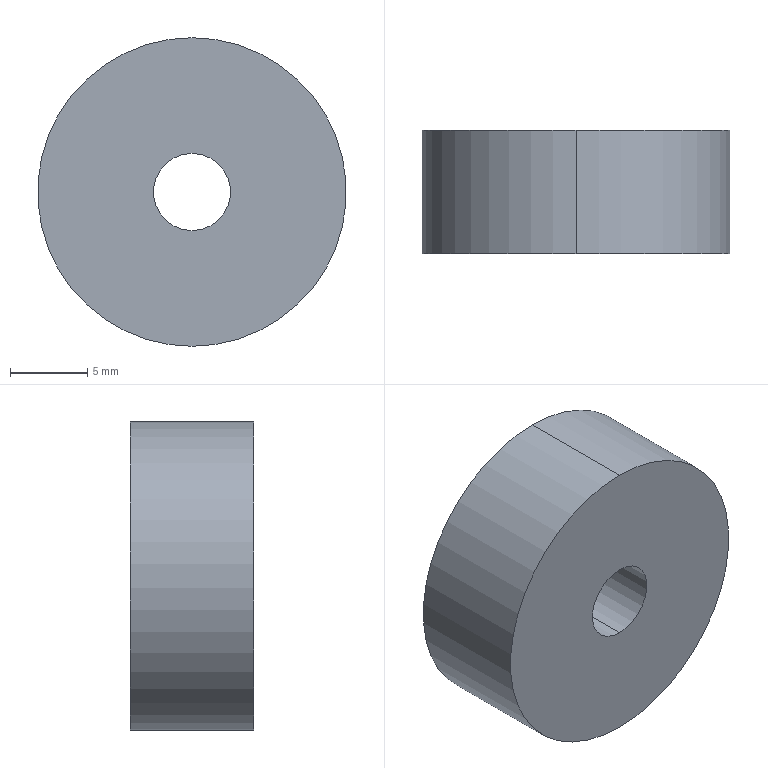Part | SolidWorks | features Extrusion 1 | 1 solid | 6 faces | box 20 x 8 x 20 mm | volume 2356 mm3 | cylinder 4 | plane 2 | commonest cylinder face diameters 5 x2 20 x2
STEP:
#1=CARTESIAN_POINT('',(0.,8.,-2.5));
#2=VERTEX_POINT('',#1);
#3=CARTESIAN_POINT('',(0.,8.,2.5));
#4=VERTEX_POINT('',#3);
#5=CARTESIAN_POINT('',(0.,8.,0.));
#6=DIRECTION('',(0.,1.,0.));
#7=DIRECTION('',(0.,0.,1.));
#8=AXIS2_PLACEMENT_3D('',#5,#6,#7);
#9=CIRCLE('',#8,2.5);
#10=EDGE_CURVE('',#2,#4,#9,.T.);
#11=ORIENTED_EDGE('',*,*,#10,.T.);
#12=CARTESIAN_POINT('',(0.,0.,2.5));
#13=VERTEX_POINT('',#12);
#14=CARTESIAN_POINT('',(0.,8.,2.5));
#15=DIRECTION('',(0.,-1.,0.));
#16=VECTOR('',#15,1000.);
#17=LINE('',#14,#16);
#18=EDGE_CURVE('',#4,#13,#17,.T.);
#19=ORIENTED_EDGE('',*,*,#18,.T.);
#20=CARTESIAN_POINT('',(0.,0.,-2.5));
#21=VERTEX_POINT('',#20);
#22=CARTESIAN_POINT('',(0.,0.,0.));
#23=DIRECTION('',(0.,1.,0.));
#24=DIRECTION('',(0.,0.,1.));
#25=AXIS2_PLACEMENT_3D('',#22,#23,#24);
#26=CIRCLE('',#25,2.5);
#27=EDGE_CURVE('',#21,#13,#26,.T.);
#28=ORIENTED_EDGE('',*,*,#27,.F.);
#29=CARTESIAN_POINT('',(0.,8.,-2.5));
#30=DIRECTION('',(0.,-1.,0.));
#31=VECTOR('',#30,1000.);
#32=LINE('',#29,#31);
#33=EDGE_CURVE('',#2,#21,#32,.T.);
#34=ORIENTED_EDGE('',*,*,#33,.F.);
#35=EDGE_LOOP('',(#11,#19,#28,#34));
#36=FACE_OUTER_BOUND('',#35,.T.);
#37=CARTESIAN_POINT('',(0.,8.,0.));
#38=DIRECTION('',(0.,-1.,0.));
#39=DIRECTION('',(0.,0.,-1.));
#40=AXIS2_PLACEMENT_3D('',#37,#38,#39);
#41=CYLINDRICAL_SURFACE('',#40,2.5);
#42=ADVANCED_FACE('',(#36),#41,.F.);
#43=CARTESIAN_POINT('',(0.,8.,10.));
#44=VERTEX_POINT('',#43);
#45=CARTESIAN_POINT('',(0.,8.,-10.));
#46=VERTEX_POINT('',#45);
#47=CARTESIAN_POINT('',(0.,8.,0.));
#48=DIRECTION('',(0.,1.,0.));
#49=DIRECTION('',(0.,0.,1.));
#50=AXIS2_PLACEMENT_3D('',#47,#48,#49);
#51=CIRCLE('',#50,10.);
#52=EDGE_CURVE('',#44,#46,#51,.T.);
#53=ORIENTED_EDGE('',*,*,#52,.F.);
#54=CARTESIAN_POINT('',(0.,0.,10.));
#55=VERTEX_POINT('',#54);
#56=CARTESIAN_POINT('',(0.,8.,10.));
#57=DIRECTION('',(0.,-1.,0.));
#58=VECTOR('',#57,1000.);
#59=LINE('',#56,#58);
#60=EDGE_CURVE('',#44,#55,#59,.T.);
#61=ORIENTED_EDGE('',*,*,#60,.T.);
#62=CARTESIAN_POINT('',(0.,0.,-10.));
#63=VERTEX_POINT('',#62);
#64=CARTESIAN_POINT('',(0.,0.,0.));
#65=DIRECTION('',(0.,1.,0.));
#66=DIRECTION('',(0.,0.,1.));
#67=AXIS2_PLACEMENT_3D('',#64,#65,#66);
#68=CIRCLE('',#67,10.);
#69=EDGE_CURVE('',#55,#63,#68,.T.);
#70=ORIENTED_EDGE('',*,*,#69,.T.);
#71=CARTESIAN_POINT('',(0.,8.,-10.));
#72=DIRECTION('',(0.,-1.,0.));
#73=VECTOR('',#72,1000.);
#74=LINE('',#71,#73);
#75=EDGE_CURVE('',#46,#63,#74,.T.);
#76=ORIENTED_EDGE('',*,*,#75,.F.);
#77=EDGE_LOOP('',(#53,#61,#70,#76));
#78=FACE_OUTER_BOUND('',#77,.T.);
#79=CARTESIAN_POINT('',(0.,8.,0.));
#80=DIRECTION('',(0.,-1.,0.));
#81=DIRECTION('',(0.,0.,-1.));
#82=AXIS2_PLACEMENT_3D('',#79,#80,#81);
#83=CYLINDRICAL_SURFACE('',#82,10.);
#84=ADVANCED_FACE('',(#78),#83,.T.);
#85=CARTESIAN_POINT('',(0.,8.,0.));
#86=DIRECTION('',(0.,1.,0.));
#87=DIRECTION('',(0.,0.,1.));
#88=AXIS2_PLACEMENT_3D('',#85,#86,#87);
#89=CIRCLE('',#88,10.);
#90=EDGE_CURVE('',#46,#44,#89,.T.);
#91=ORIENTED_EDGE('',*,*,#90,.T.);
#92=ORIENTED_EDGE('',*,*,#52,.T.);
#93=EDGE_LOOP('',(#91,#92));
#94=FACE_OUTER_BOUND('',#93,.T.);
#95=ORIENTED_EDGE('',*,*,#10,.F.);
#96=CARTESIAN_POINT('',(0.,8.,0.));
#97=DIRECTION('',(0.,1.,0.));
#98=DIRECTION('',(0.,0.,1.));
#99=AXIS2_PLACEMENT_3D('',#96,#97,#98);
#100=CIRCLE('',#99,2.5);
#101=EDGE_CURVE('',#4,#2,#100,.T.);
#102=ORIENTED_EDGE('',*,*,#101,.F.);
#103=EDGE_LOOP('',(#95,#102));
#104=FACE_BOUND('',#103,.T.);
#105=CARTESIAN_POINT('',(0.,8.,0.));
#106=DIRECTION('',(0.,1.,0.));
#107=DIRECTION('',(0.,0.,1.));
#108=AXIS2_PLACEMENT_3D('',#105,#106,#107);
#109=PLANE('',#108);
#110=ADVANCED_FACE('',(#94,#104),#109,.T.);
#111=CARTESIAN_POINT('',(0.,0.,0.));
#112=DIRECTION('',(0.,1.,0.));
#113=DIRECTION('',(0.,0.,1.));
#114=AXIS2_PLACEMENT_3D('',#111,#112,#113);
#115=CIRCLE('',#114,10.);
#116=EDGE_CURVE('',#63,#55,#115,.T.);
#117=ORIENTED_EDGE('',*,*,#116,.F.);
#118=ORIENTED_EDGE('',*,*,#69,.F.);
#119=EDGE_LOOP('',(#117,#118));
#120=FACE_OUTER_BOUND('',#119,.T.);
#121=ORIENTED_EDGE('',*,*,#27,.T.);
#122=CARTESIAN_POINT('',(0.,0.,0.));
#123=DIRECTION('',(0.,1.,0.));
#124=DIRECTION('',(0.,0.,1.));
#125=AXIS2_PLACEMENT_3D('',#122,#123,#124);
#126=CIRCLE('',#125,2.5);
#127=EDGE_CURVE('',#13,#21,#126,.T.);
#128=ORIENTED_EDGE('',*,*,#127,.T.);
#129=EDGE_LOOP('',(#121,#128));
#130=FACE_BOUND('',#129,.T.);
#131=CARTESIAN_POINT('',(0.,0.,0.));
#132=DIRECTION('',(0.,1.,0.));
#133=DIRECTION('',(0.,0.,1.));
#134=AXIS2_PLACEMENT_3D('',#131,#132,#133);
#135=PLANE('',#134);
#136=ADVANCED_FACE('',(#120,#130),#135,.F.);
#137=ORIENTED_EDGE('',*,*,#60,.F.);
#138=ORIENTED_EDGE('',*,*,#90,.F.);
#139=ORIENTED_EDGE('',*,*,#75,.T.);
#140=ORIENTED_EDGE('',*,*,#116,.T.);
#141=EDGE_LOOP('',(#137,#138,#139,#140));
#142=FACE_OUTER_BOUND('',#141,.T.);
#143=CARTESIAN_POINT('',(0.,8.,0.));
#144=DIRECTION('',(0.,-1.,0.));
#145=DIRECTION('',(0.,0.,-1.));
#146=AXIS2_PLACEMENT_3D('',#143,#144,#145);
#147=CYLINDRICAL_SURFACE('',#146,10.);
#148=ADVANCED_FACE('',(#142),#147,.T.);
#149=ORIENTED_EDGE('',*,*,#18,.F.);
#150=ORIENTED_EDGE('',*,*,#101,.T.);
#151=ORIENTED_EDGE('',*,*,#33,.T.);
#152=ORIENTED_EDGE('',*,*,#127,.F.);
#153=EDGE_LOOP('',(#149,#150,#151,#152));
#154=FACE_OUTER_BOUND('',#153,.T.);
#155=CARTESIAN_POINT('',(0.,8.,0.));
#156=DIRECTION('',(0.,-1.,0.));
#157=DIRECTION('',(0.,0.,-1.));
#158=AXIS2_PLACEMENT_3D('',#155,#156,#157);
#159=CYLINDRICAL_SURFACE('',#158,2.5);
#160=ADVANCED_FACE('',(#154),#159,.F.);
#161=CLOSED_SHELL('',(#42,#84,#110,#136,#148,#160));
#162=MANIFOLD_SOLID_BREP('',#161);
#163=CARTESIAN_POINT('',(0.,0.,0.));
#164=DIRECTION('',(0.,0.,1.));
#165=DIRECTION('',(1.,0.,0.));
#166=AXIS2_PLACEMENT_3D('',#163,#164,#165);
#167=(LENGTH_UNIT()NAMED_UNIT(*)SI_UNIT(.MILLI.,.METRE.));
#168=UNCERTAINTY_MEASURE_WITH_UNIT(LENGTH_MEASURE(0.00001),#167,'','');
#169=(NAMED_UNIT(*)PLANE_ANGLE_UNIT()SI_UNIT($,.RADIAN.));
#170=(NAMED_UNIT(*)SI_UNIT($,.STERADIAN.)SOLID_ANGLE_UNIT());
#171=(GEOMETRIC_REPRESENTATION_CONTEXT(3)GLOBAL_UNCERTAINTY_ASSIGNED_CONTEXT((#168))GLOBAL_UNIT_ASSIGNED_CONTEXT((#167,#169,#170))REPRESENTATION_CONTEXT('',''));
#172=ADVANCED_BREP_SHAPE_REPRESENTATION('',(#162,#166),#171);